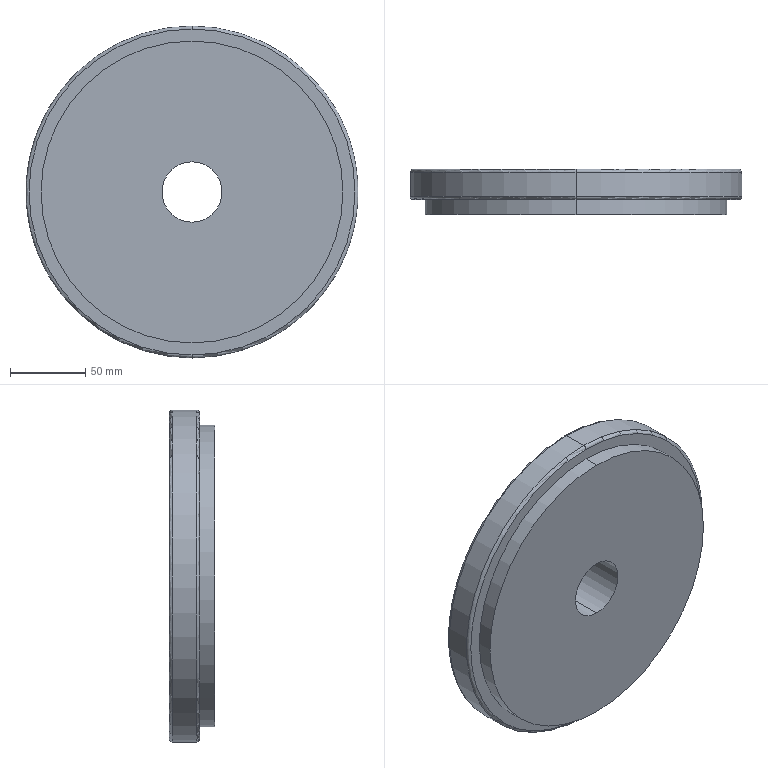Part | SolidWorks | features ICE 2, Extrusion 1, Fillet 1, HoleWzd 1, SketchPattern 1 | 1 solid | 29 faces | box 220 x 30 x 220 mm | volume 1035187 mm3 | cylinder 14 | cone 8 | torus 4 | plane 3 | commonest cylinder face diameters 3.3 x8 40 x2 200 x2 220 x2
STEP:
#1=CARTESIAN_POINT('',(0.,28.,-110.));
#2=VERTEX_POINT('',#1);
#3=CARTESIAN_POINT('',(0.,28.,110.));
#4=VERTEX_POINT('',#3);
#5=CARTESIAN_POINT('',(0.,28.,0.));
#6=DIRECTION('',(0.,-1.,0.));
#7=DIRECTION('',(0.,0.,1.));
#8=AXIS2_PLACEMENT_3D('',#5,#6,#7);
#9=CIRCLE('',#8,110.);
#10=EDGE_CURVE('',#2,#4,#9,.T.);
#11=ORIENTED_EDGE('',*,*,#10,.F.);
#12=CARTESIAN_POINT('',(0.,30.,-108.));
#13=VERTEX_POINT('',#12);
#14=CARTESIAN_POINT('',(0.,28.,-108.));
#15=DIRECTION('',(1.,0.,0.));
#16=DIRECTION('',(0.,0.,-1.));
#17=AXIS2_PLACEMENT_3D('',#14,#15,#16);
#18=CIRCLE('',#17,2.);
#19=EDGE_CURVE('',#2,#13,#18,.T.);
#20=ORIENTED_EDGE('',*,*,#19,.T.);
#21=CARTESIAN_POINT('',(0.,30.,108.));
#22=VERTEX_POINT('',#21);
#23=CARTESIAN_POINT('',(0.,30.,0.));
#24=DIRECTION('',(0.,1.,0.));
#25=DIRECTION('',(0.,0.,1.));
#26=AXIS2_PLACEMENT_3D('',#23,#24,#25);
#27=CIRCLE('',#26,108.);
#28=EDGE_CURVE('',#22,#13,#27,.T.);
#29=ORIENTED_EDGE('',*,*,#28,.F.);
#30=CARTESIAN_POINT('',(0.,28.,108.));
#31=DIRECTION('',(-1.,0.,0.));
#32=DIRECTION('',(0.,0.,1.));
#33=AXIS2_PLACEMENT_3D('',#30,#31,#32);
#34=CIRCLE('',#33,2.);
#35=EDGE_CURVE('',#4,#22,#34,.T.);
#36=ORIENTED_EDGE('',*,*,#35,.F.);
#37=EDGE_LOOP('',(#11,#20,#29,#36));
#38=FACE_OUTER_BOUND('',#37,.T.);
#39=CARTESIAN_POINT('',(0.,28.,0.));
#40=DIRECTION('',(0.,1.,0.));
#41=DIRECTION('',(0.,0.,1.));
#42=AXIS2_PLACEMENT_3D('',#39,#40,#41);
#43=TOROIDAL_SURFACE('',#42,108.,2.);
#44=ADVANCED_FACE('',(#38),#43,.T.);
#45=CARTESIAN_POINT('',(0.,10.,-108.));
#46=VERTEX_POINT('',#45);
#47=CARTESIAN_POINT('',(0.,10.,108.));
#48=VERTEX_POINT('',#47);
#49=CARTESIAN_POINT('',(0.,10.,0.));
#50=DIRECTION('',(0.,-1.,0.));
#51=DIRECTION('',(0.,0.,1.));
#52=AXIS2_PLACEMENT_3D('',#49,#50,#51);
#53=CIRCLE('',#52,108.);
#54=EDGE_CURVE('',#46,#48,#53,.T.);
#55=ORIENTED_EDGE('',*,*,#54,.F.);
#56=CARTESIAN_POINT('',(0.,12.,-110.));
#57=VERTEX_POINT('',#56);
#58=CARTESIAN_POINT('',(0.,12.,-108.));
#59=DIRECTION('',(1.,0.,0.));
#60=DIRECTION('',(0.,0.,-1.));
#61=AXIS2_PLACEMENT_3D('',#58,#59,#60);
#62=CIRCLE('',#61,2.);
#63=EDGE_CURVE('',#46,#57,#62,.T.);
#64=ORIENTED_EDGE('',*,*,#63,.T.);
#65=CARTESIAN_POINT('',(0.,12.,110.));
#66=VERTEX_POINT('',#65);
#67=CARTESIAN_POINT('',(0.,12.,0.));
#68=DIRECTION('',(0.,1.,0.));
#69=DIRECTION('',(0.,0.,1.));
#70=AXIS2_PLACEMENT_3D('',#67,#68,#69);
#71=CIRCLE('',#70,110.);
#72=EDGE_CURVE('',#66,#57,#71,.T.);
#73=ORIENTED_EDGE('',*,*,#72,.F.);
#74=CARTESIAN_POINT('',(0.,12.,108.));
#75=DIRECTION('',(-1.,0.,0.));
#76=DIRECTION('',(0.,0.,1.));
#77=AXIS2_PLACEMENT_3D('',#74,#75,#76);
#78=CIRCLE('',#77,2.);
#79=EDGE_CURVE('',#48,#66,#78,.T.);
#80=ORIENTED_EDGE('',*,*,#79,.F.);
#81=EDGE_LOOP('',(#55,#64,#73,#80));
#82=FACE_OUTER_BOUND('',#81,.T.);
#83=CARTESIAN_POINT('',(0.,12.,0.));
#84=DIRECTION('',(0.,1.,0.));
#85=DIRECTION('',(0.,0.,1.));
#86=AXIS2_PLACEMENT_3D('',#83,#84,#85);
#87=TOROIDAL_SURFACE('',#86,108.,2.);
#88=ADVANCED_FACE('',(#82),#87,.T.);
#89=CARTESIAN_POINT('',(-22.707,19.9,-12.11));
#90=VERTEX_POINT('',#89);
#91=CARTESIAN_POINT('',(-22.707,19.9,-8.81));
#92=VERTEX_POINT('',#91);
#93=CARTESIAN_POINT('',(-22.707,19.9,-10.46));
#94=DIRECTION('',(0.,1.,0.));
#95=DIRECTION('',(0.,0.,1.));
#96=AXIS2_PLACEMENT_3D('',#93,#94,#95);
#97=CIRCLE('',#96,1.65);
#98=EDGE_CURVE('',#90,#92,#97,.T.);
#99=ORIENTED_EDGE('',*,*,#98,.F.);
#100=CARTESIAN_POINT('',(-22.707,30.,-12.11));
#101=VERTEX_POINT('',#100);
#102=CARTESIAN_POINT('',(-22.707,30.,-12.11));
#103=DIRECTION('',(0.,1.,0.));
#104=VECTOR('',#103,1000.);
#105=LINE('',#102,#104);
#106=EDGE_CURVE('',#90,#101,#105,.T.);
#107=ORIENTED_EDGE('',*,*,#106,.T.);
#108=CARTESIAN_POINT('',(-22.707,30.,-8.81));
#109=VERTEX_POINT('',#108);
#110=CARTESIAN_POINT('',(-22.707,30.,-10.46));
#111=DIRECTION('',(0.,1.,0.));
#112=DIRECTION('',(0.,0.,1.));
#113=AXIS2_PLACEMENT_3D('',#110,#111,#112);
#114=CIRCLE('',#113,1.65);
#115=EDGE_CURVE('',#101,#109,#114,.T.);
#116=ORIENTED_EDGE('',*,*,#115,.T.);
#117=CARTESIAN_POINT('',(-22.707,30.,-8.81));
#118=DIRECTION('',(0.,1.,0.));
#119=VECTOR('',#118,1000.);
#120=LINE('',#117,#119);
#121=EDGE_CURVE('',#92,#109,#120,.T.);
#122=ORIENTED_EDGE('',*,*,#121,.F.);
#123=EDGE_LOOP('',(#99,#107,#116,#122));
#124=FACE_OUTER_BOUND('',#123,.T.);
#125=CARTESIAN_POINT('',(-22.707,30.,-10.46));
#126=DIRECTION('',(0.,1.,0.));
#127=DIRECTION('',(0.,0.,1.));
#128=AXIS2_PLACEMENT_3D('',#125,#126,#127);
#129=CYLINDRICAL_SURFACE('',#128,1.65);
#130=ADVANCED_FACE('',(#124),#129,.F.);
#131=CARTESIAN_POINT('',(-22.707,18.909,-10.46));
#132=VERTEX_POINT('',#131);
#133=CARTESIAN_POINT('',(-22.707,19.9,-8.81));
#134=DIRECTION('',(0.,0.515,0.8572));
#135=VECTOR('',#134,1000.);
#136=LINE('',#133,#135);
#137=EDGE_CURVE('',#132,#92,#136,.T.);
#138=ORIENTED_EDGE('',*,*,#137,.F.);
#139=CARTESIAN_POINT('',(-22.707,19.9,-12.11));
#140=DIRECTION('',(0.,0.515,-0.8572));
#141=VECTOR('',#140,1000.);
#142=LINE('',#139,#141);
#143=EDGE_CURVE('',#132,#90,#142,.T.);
#144=ORIENTED_EDGE('',*,*,#143,.T.);
#145=ORIENTED_EDGE('',*,*,#98,.T.);
#146=EDGE_LOOP('',(#138,#144,#145));
#147=FACE_OUTER_BOUND('',#146,.T.);
#148=CARTESIAN_POINT('',(-22.707,19.9,-10.46));
#149=DIRECTION('',(0.,1.,0.));
#150=DIRECTION('',(0.,0.,1.));
#151=AXIS2_PLACEMENT_3D('',#148,#149,#150);
#152=CONICAL_SURFACE('',#151,1.65,1.03);
#153=ADVANCED_FACE('',(#147),#152,.F.);
#154=CARTESIAN_POINT('',(-7.031,19.9,30.343));
#155=VERTEX_POINT('',#154);
#156=CARTESIAN_POINT('',(-7.031,19.9,33.643));
#157=VERTEX_POINT('',#156);
#158=CARTESIAN_POINT('',(-7.031,19.9,31.993));
#159=DIRECTION('',(0.,1.,0.));
#160=DIRECTION('',(0.,0.,1.));
#161=AXIS2_PLACEMENT_3D('',#158,#159,#160);
#162=CIRCLE('',#161,1.65);
#163=EDGE_CURVE('',#155,#157,#162,.T.);
#164=ORIENTED_EDGE('',*,*,#163,.F.);
#165=CARTESIAN_POINT('',(-7.031,30.,30.343));
#166=VERTEX_POINT('',#165);
#167=CARTESIAN_POINT('',(-7.031,30.,30.343));
#168=DIRECTION('',(0.,1.,0.));
#169=VECTOR('',#168,1000.);
#170=LINE('',#167,#169);
#171=EDGE_CURVE('',#155,#166,#170,.T.);
#172=ORIENTED_EDGE('',*,*,#171,.T.);
#173=CARTESIAN_POINT('',(-7.031,30.,33.643));
#174=VERTEX_POINT('',#173);
#175=CARTESIAN_POINT('',(-7.031,30.,31.993));
#176=DIRECTION('',(0.,1.,0.));
#177=DIRECTION('',(0.,0.,1.));
#178=AXIS2_PLACEMENT_3D('',#175,#176,#177);
#179=CIRCLE('',#178,1.65);
#180=EDGE_CURVE('',#166,#174,#179,.T.);
#181=ORIENTED_EDGE('',*,*,#180,.T.);
#182=CARTESIAN_POINT('',(-7.031,30.,33.643));
#183=DIRECTION('',(0.,1.,0.));
#184=VECTOR('',#183,1000.);
#185=LINE('',#182,#184);
#186=EDGE_CURVE('',#157,#174,#185,.T.);
#187=ORIENTED_EDGE('',*,*,#186,.F.);
#188=EDGE_LOOP('',(#164,#172,#181,#187));
#189=FACE_OUTER_BOUND('',#188,.T.);
#190=CARTESIAN_POINT('',(-7.031,30.,31.993));
#191=DIRECTION('',(0.,1.,0.));
#192=DIRECTION('',(0.,0.,1.));
#193=AXIS2_PLACEMENT_3D('',#190,#191,#192);
#194=CYLINDRICAL_SURFACE('',#193,1.65);
#195=ADVANCED_FACE('',(#189),#194,.F.);
#196=CARTESIAN_POINT('',(-7.031,18.909,31.993));
#197=VERTEX_POINT('',#196);
#198=CARTESIAN_POINT('',(-7.031,19.9,33.643));
#199=DIRECTION('',(0.,0.515,0.8572));
#200=VECTOR('',#199,1000.);
#201=LINE('',#198,#200);
#202=EDGE_CURVE('',#197,#157,#201,.T.);
#203=ORIENTED_EDGE('',*,*,#202,.F.);
#204=CARTESIAN_POINT('',(-7.031,19.9,30.343));
#205=DIRECTION('',(0.,0.515,-0.8572));
#206=VECTOR('',#205,1000.);
#207=LINE('',#204,#206);
#208=EDGE_CURVE('',#197,#155,#207,.T.);
#209=ORIENTED_EDGE('',*,*,#208,.T.);
#210=ORIENTED_EDGE('',*,*,#163,.T.);
#211=EDGE_LOOP('',(#203,#209,#210));
#212=FACE_OUTER_BOUND('',#211,.T.);
#213=CARTESIAN_POINT('',(-7.031,19.9,31.993));
#214=DIRECTION('',(0.,1.,0.));
#215=DIRECTION('',(0.,0.,1.));
#216=AXIS2_PLACEMENT_3D('',#213,#214,#215);
#217=CONICAL_SURFACE('',#216,1.65,1.03);
#218=ADVANCED_FACE('',(#212),#217,.F.);
#219=CARTESIAN_POINT('',(35.422,19.9,14.668));
#220=VERTEX_POINT('',#219);
#221=CARTESIAN_POINT('',(35.422,19.9,17.968));
#222=VERTEX_POINT('',#221);
#223=CARTESIAN_POINT('',(35.422,19.9,16.318));
#224=DIRECTION('',(0.,1.,0.));
#225=DIRECTION('',(0.,0.,1.));
#226=AXIS2_PLACEMENT_3D('',#223,#224,#225);
#227=CIRCLE('',#226,1.65);
#228=EDGE_CURVE('',#220,#222,#227,.T.);
#229=ORIENTED_EDGE('',*,*,#228,.F.);
#230=CARTESIAN_POINT('',(35.422,30.,14.668));
#231=VERTEX_POINT('',#230);
#232=CARTESIAN_POINT('',(35.422,30.,14.668));
#233=DIRECTION('',(0.,1.,0.));
#234=VECTOR('',#233,1000.);
#235=LINE('',#232,#234);
#236=EDGE_CURVE('',#220,#231,#235,.T.);
#237=ORIENTED_EDGE('',*,*,#236,.T.);
#238=CARTESIAN_POINT('',(35.422,30.,17.968));
#239=VERTEX_POINT('',#238);
#240=CARTESIAN_POINT('',(35.422,30.,16.318));
#241=DIRECTION('',(0.,1.,0.));
#242=DIRECTION('',(0.,0.,1.));
#243=AXIS2_PLACEMENT_3D('',#240,#241,#242);
#244=CIRCLE('',#243,1.65);
#245=EDGE_CURVE('',#231,#239,#244,.T.);
#246=ORIENTED_EDGE('',*,*,#245,.T.);
#247=CARTESIAN_POINT('',(35.422,30.,17.968));
#248=DIRECTION('',(0.,1.,0.));
#249=VECTOR('',#248,1000.);
#250=LINE('',#247,#249);
#251=EDGE_CURVE('',#222,#239,#250,.T.);
#252=ORIENTED_EDGE('',*,*,#251,.F.);
#253=EDGE_LOOP('',(#229,#237,#246,#252));
#254=FACE_OUTER_BOUND('',#253,.T.);
#255=CARTESIAN_POINT('',(35.422,30.,16.318));
#256=DIRECTION('',(0.,1.,0.));
#257=DIRECTION('',(0.,0.,1.));
#258=AXIS2_PLACEMENT_3D('',#255,#256,#257);
#259=CYLINDRICAL_SURFACE('',#258,1.65);
#260=ADVANCED_FACE('',(#254),#259,.F.);
#261=CARTESIAN_POINT('',(35.422,18.909,16.318));
#262=VERTEX_POINT('',#261);
#263=CARTESIAN_POINT('',(35.422,19.9,17.968));
#264=DIRECTION('',(0.,0.515,0.8572));
#265=VECTOR('',#264,1000.);
#266=LINE('',#263,#265);
#267=EDGE_CURVE('',#262,#222,#266,.T.);
#268=ORIENTED_EDGE('',*,*,#267,.F.);
#269=CARTESIAN_POINT('',(35.422,19.9,14.668));
#270=DIRECTION('',(0.,0.515,-0.8572));
#271=VECTOR('',#270,1000.);
#272=LINE('',#269,#271);
#273=EDGE_CURVE('',#262,#220,#272,.T.);
#274=ORIENTED_EDGE('',*,*,#273,.T.);
#275=ORIENTED_EDGE('',*,*,#228,.T.);
#276=EDGE_LOOP('',(#268,#274,#275));
#277=FACE_OUTER_BOUND('',#276,.T.);
#278=CARTESIAN_POINT('',(35.422,19.9,16.318));
#279=DIRECTION('',(0.,1.,0.));
#280=DIRECTION('',(0.,0.,1.));
#281=AXIS2_PLACEMENT_3D('',#278,#279,#280);
#282=CONICAL_SURFACE('',#281,1.65,1.03);
#283=ADVANCED_FACE('',(#277),#282,.F.);
#284=CARTESIAN_POINT('',(19.747,19.9,-27.786));
#285=VERTEX_POINT('',#284);
#286=CARTESIAN_POINT('',(19.747,19.9,-24.486));
#287=VERTEX_POINT('',#286);
#288=CARTESIAN_POINT('',(19.747,19.9,-26.136));
#289=DIRECTION('',(0.,1.,0.));
#290=DIRECTION('',(0.,0.,1.));
#291=AXIS2_PLACEMENT_3D('',#288,#289,#290);
#292=CIRCLE('',#291,1.65);
#293=EDGE_CURVE('',#285,#287,#292,.T.);
#294=ORIENTED_EDGE('',*,*,#293,.F.);
#295=CARTESIAN_POINT('',(19.747,30.,-27.786));
#296=VERTEX_POINT('',#295);
#297=CARTESIAN_POINT('',(19.747,30.,-27.786));
#298=DIRECTION('',(0.,1.,0.));
#299=VECTOR('',#298,1000.);
#300=LINE('',#297,#299);
#301=EDGE_CURVE('',#285,#296,#300,.T.);
#302=ORIENTED_EDGE('',*,*,#301,.T.);
#303=CARTESIAN_POINT('',(19.747,30.,-24.486));
#304=VERTEX_POINT('',#303);
#305=CARTESIAN_POINT('',(19.747,30.,-26.136));
#306=DIRECTION('',(0.,1.,0.));
#307=DIRECTION('',(0.,0.,1.));
#308=AXIS2_PLACEMENT_3D('',#305,#306,#307);
#309=CIRCLE('',#308,1.65);
#310=EDGE_CURVE('',#296,#304,#309,.T.);
#311=ORIENTED_EDGE('',*,*,#310,.T.);
#312=CARTESIAN_POINT('',(19.747,30.,-24.486));
#313=DIRECTION('',(0.,1.,0.));
#314=VECTOR('',#313,1000.);
#315=LINE('',#312,#314);
#316=EDGE_CURVE('',#287,#304,#315,.T.);
#317=ORIENTED_EDGE('',*,*,#316,.F.);
#318=EDGE_LOOP('',(#294,#302,#311,#317));
#319=FACE_OUTER_BOUND('',#318,.T.);
#320=CARTESIAN_POINT('',(19.747,30.,-26.136));
#321=DIRECTION('',(0.,1.,0.));
#322=DIRECTION('',(0.,0.,1.));
#323=AXIS2_PLACEMENT_3D('',#320,#321,#322);
#324=CYLINDRICAL_SURFACE('',#323,1.65);
#325=ADVANCED_FACE('',(#319),#324,.F.);
#326=CARTESIAN_POINT('',(19.747,18.909,-26.136));
#327=VERTEX_POINT('',#326);
#328=CARTESIAN_POINT('',(19.747,19.9,-24.486));
#329=DIRECTION('',(0.,0.515,0.8572));
#330=VECTOR('',#329,1000.);
#331=LINE('',#328,#330);
#332=EDGE_CURVE('',#327,#287,#331,.T.);
#333=ORIENTED_EDGE('',*,*,#332,.F.);
#334=CARTESIAN_POINT('',(19.747,19.9,-27.786));
#335=DIRECTION('',(0.,0.515,-0.8572));
#336=VECTOR('',#335,1000.);
#337=LINE('',#334,#336);
#338=EDGE_CURVE('',#327,#285,#337,.T.);
#339=ORIENTED_EDGE('',*,*,#338,.T.);
#340=ORIENTED_EDGE('',*,*,#293,.T.);
#341=EDGE_LOOP('',(#333,#339,#340));
#342=FACE_OUTER_BOUND('',#341,.T.);
#343=CARTESIAN_POINT('',(19.747,19.9,-26.136));
#344=DIRECTION('',(0.,1.,0.));
#345=DIRECTION('',(0.,0.,1.));
#346=AXIS2_PLACEMENT_3D('',#343,#344,#345);
#347=CONICAL_SURFACE('',#346,1.65,1.03);
#348=ADVANCED_FACE('',(#342),#347,.F.);
#349=CARTESIAN_POINT('',(0.,0.,-20.));
#350=VERTEX_POINT('',#349);
#351=CARTESIAN_POINT('',(0.,0.,20.));
#352=VERTEX_POINT('',#351);
#353=CARTESIAN_POINT('',(0.,0.,0.));
#354=DIRECTION('',(0.,1.,0.));
#355=DIRECTION('',(0.,0.,1.));
#356=AXIS2_PLACEMENT_3D('',#353,#354,#355);
#357=CIRCLE('',#356,20.);
#358=EDGE_CURVE('',#350,#352,#357,.T.);
#359=ORIENTED_EDGE('',*,*,#358,.F.);
#360=CARTESIAN_POINT('',(0.,30.,-20.));
#361=VERTEX_POINT('',#360);
#362=CARTESIAN_POINT('',(0.,0.,-20.));
#363=DIRECTION('',(0.,1.,0.));
#364=VECTOR('',#363,1000.);
#365=LINE('',#362,#364);
#366=EDGE_CURVE('',#350,#361,#365,.T.);
#367=ORIENTED_EDGE('',*,*,#366,.T.);
#368=CARTESIAN_POINT('',(0.,30.,20.));
#369=VERTEX_POINT('',#368);
#370=CARTESIAN_POINT('',(0.,30.,0.));
#371=DIRECTION('',(0.,1.,0.));
#372=DIRECTION('',(0.,0.,1.));
#373=AXIS2_PLACEMENT_3D('',#370,#371,#372);
#374=CIRCLE('',#373,20.);
#375=EDGE_CURVE('',#361,#369,#374,.T.);
#376=ORIENTED_EDGE('',*,*,#375,.T.);
#377=CARTESIAN_POINT('',(0.,0.,20.));
#378=DIRECTION('',(0.,1.,0.));
#379=VECTOR('',#378,1000.);
#380=LINE('',#377,#379);
#381=EDGE_CURVE('',#352,#369,#380,.T.);
#382=ORIENTED_EDGE('',*,*,#381,.F.);
#383=EDGE_LOOP('',(#359,#367,#376,#382));
#384=FACE_OUTER_BOUND('',#383,.T.);
#385=CARTESIAN_POINT('',(0.,0.,0.));
#386=DIRECTION('',(0.,1.,0.));
#387=DIRECTION('',(0.,0.,1.));
#388=AXIS2_PLACEMENT_3D('',#385,#386,#387);
#389=CYLINDRICAL_SURFACE('',#388,20.);
#390=ADVANCED_FACE('',(#384),#389,.F.);
#391=ORIENTED_EDGE('',*,*,#10,.T.);
#392=CARTESIAN_POINT('',(0.,30.,110.));
#393=DIRECTION('',(0.,-1.,0.));
#394=VECTOR('',#393,1000.);
#395=LINE('',#392,#394);
#396=EDGE_CURVE('',#4,#66,#395,.T.);
#397=ORIENTED_EDGE('',*,*,#396,.T.);
#398=ORIENTED_EDGE('',*,*,#72,.T.);
#399=CARTESIAN_POINT('',(0.,30.,-110.));
#400=DIRECTION('',(0.,-1.,0.));
#401=VECTOR('',#400,1000.);
#402=LINE('',#399,#401);
#403=EDGE_CURVE('',#2,#57,#402,.T.);
#404=ORIENTED_EDGE('',*,*,#403,.F.);
#405=EDGE_LOOP('',(#391,#397,#398,#404));
#406=FACE_OUTER_BOUND('',#405,.T.);
#407=CARTESIAN_POINT('',(0.,30.,0.));
#408=DIRECTION('',(0.,-1.,0.));
#409=DIRECTION('',(0.,0.,-1.));
#410=AXIS2_PLACEMENT_3D('',#407,#408,#409);
#411=CYLINDRICAL_SURFACE('',#410,110.);
#412=ADVANCED_FACE('',(#406),#411,.T.);
#413=CARTESIAN_POINT('',(0.,10.,100.));
#414=VERTEX_POINT('',#413);
#415=CARTESIAN_POINT('',(0.,10.,-100.));
#416=VERTEX_POINT('',#415);
#417=CARTESIAN_POINT('',(0.,10.,0.));
#418=DIRECTION('',(0.,1.,0.));
#419=DIRECTION('',(0.,0.,1.));
#420=AXIS2_PLACEMENT_3D('',#417,#418,#419);
#421=CIRCLE('',#420,100.);
#422=EDGE_CURVE('',#414,#416,#421,.T.);
#423=ORIENTED_EDGE('',*,*,#422,.F.);
#424=CARTESIAN_POINT('',(0.,0.,100.));
#425=VERTEX_POINT('',#424);
#426=CARTESIAN_POINT('',(0.,10.,100.));
#427=DIRECTION('',(0.,-1.,0.));
#428=VECTOR('',#427,1000.);
#429=LINE('',#426,#428);
#430=EDGE_CURVE('',#414,#425,#429,.T.);
#431=ORIENTED_EDGE('',*,*,#430,.T.);
#432=CARTESIAN_POINT('',(0.,0.,-100.));
#433=VERTEX_POINT('',#432);
#434=CARTESIAN_POINT('',(0.,0.,0.));
#435=DIRECTION('',(0.,1.,0.));
#436=DIRECTION('',(0.,0.,1.));
#437=AXIS2_PLACEMENT_3D('',#434,#435,#436);
#438=CIRCLE('',#437,100.);
#439=EDGE_CURVE('',#425,#433,#438,.T.);
#440=ORIENTED_EDGE('',*,*,#439,.T.);
#441=CARTESIAN_POINT('',(0.,10.,-100.));
#442=DIRECTION('',(0.,-1.,0.));
#443=VECTOR('',#442,1000.);
#444=LINE('',#441,#443);
#445=EDGE_CURVE('',#416,#433,#444,.T.);
#446=ORIENTED_EDGE('',*,*,#445,.F.);
#447=EDGE_LOOP('',(#423,#431,#440,#446));
#448=FACE_OUTER_BOUND('',#447,.T.);
#449=CARTESIAN_POINT('',(0.,10.,0.));
#450=DIRECTION('',(0.,-1.,0.));
#451=DIRECTION('',(0.,0.,-1.));
#452=AXIS2_PLACEMENT_3D('',#449,#450,#451);
#453=CYLINDRICAL_SURFACE('',#452,100.);
#454=ADVANCED_FACE('',(#448),#453,.T.);
#455=ORIENTED_EDGE('',*,*,#430,.F.);
#456=CARTESIAN_POINT('',(0.,10.,0.));
#457=DIRECTION('',(0.,1.,0.));
#458=DIRECTION('',(0.,0.,1.));
#459=AXIS2_PLACEMENT_3D('',#456,#457,#458);
#460=CIRCLE('',#459,100.);
#461=EDGE_CURVE('',#416,#414,#460,.T.);
#462=ORIENTED_EDGE('',*,*,#461,.F.);
#463=ORIENTED_EDGE('',*,*,#445,.T.);
#464=CARTESIAN_POINT('',(0.,0.,0.));
#465=DIRECTION('',(0.,1.,0.));
#466=DIRECTION('',(0.,0.,1.));
#467=AXIS2_PLACEMENT_3D('',#464,#465,#466);
#468=CIRCLE('',#467,100.);
#469=EDGE_CURVE('',#433,#425,#468,.T.);
#470=ORIENTED_EDGE('',*,*,#469,.T.);
#471=EDGE_LOOP('',(#455,#462,#463,#470));
#472=FACE_OUTER_BOUND('',#471,.T.);
#473=CARTESIAN_POINT('',(0.,10.,0.));
#474=DIRECTION('',(0.,-1.,0.));
#475=DIRECTION('',(0.,0.,-1.));
#476=AXIS2_PLACEMENT_3D('',#473,#474,#475);
#477=CYLINDRICAL_SURFACE('',#476,100.);
#478=ADVANCED_FACE('',(#472),#477,.T.);
#479=CARTESIAN_POINT('',(0.,0.,0.));
#480=DIRECTION('',(0.,1.,0.));
#481=DIRECTION('',(0.,0.,1.));
#482=AXIS2_PLACEMENT_3D('',#479,#480,#481);
#483=CIRCLE('',#482,20.);
#484=EDGE_CURVE('',#352,#350,#483,.T.);
#485=ORIENTED_EDGE('',*,*,#484,.T.);
#486=ORIENTED_EDGE('',*,*,#358,.T.);
#487=EDGE_LOOP('',(#485,#486));
#488=FACE_BOUND('',#487,.T.);
#489=ORIENTED_EDGE('',*,*,#469,.F.);
#490=ORIENTED_EDGE('',*,*,#439,.F.);
#491=EDGE_LOOP('',(#489,#490));
#492=FACE_OUTER_BOUND('',#491,.T.);
#493=CARTESIAN_POINT('',(0.,0.,0.));
#494=DIRECTION('',(0.,1.,0.));
#495=DIRECTION('',(0.,0.,1.));
#496=AXIS2_PLACEMENT_3D('',#493,#494,#495);
#497=PLANE('',#496);
#498=ADVANCED_FACE('',(#488,#492),#497,.F.);
#499=ORIENTED_EDGE('',*,*,#396,.F.);
#500=CARTESIAN_POINT('',(0.,28.,0.));
#501=DIRECTION('',(0.,-1.,0.));
#502=DIRECTION('',(0.,0.,1.));
#503=AXIS2_PLACEMENT_3D('',#500,#501,#502);
#504=CIRCLE('',#503,110.);
#505=EDGE_CURVE('',#4,#2,#504,.T.);
#506=ORIENTED_EDGE('',*,*,#505,.T.);
#507=ORIENTED_EDGE('',*,*,#403,.T.);
#508=CARTESIAN_POINT('',(0.,12.,0.));
#509=DIRECTION('',(0.,1.,0.));
#510=DIRECTION('',(0.,0.,1.));
#511=AXIS2_PLACEMENT_3D('',#508,#509,#510);
#512=CIRCLE('',#511,110.);
#513=EDGE_CURVE('',#57,#66,#512,.T.);
#514=ORIENTED_EDGE('',*,*,#513,.T.);
#515=EDGE_LOOP('',(#499,#506,#507,#514));
#516=FACE_OUTER_BOUND('',#515,.T.);
#517=CARTESIAN_POINT('',(0.,30.,0.));
#518=DIRECTION('',(0.,-1.,0.));
#519=DIRECTION('',(0.,0.,-1.));
#520=AXIS2_PLACEMENT_3D('',#517,#518,#519);
#521=CYLINDRICAL_SURFACE('',#520,110.);
#522=ADVANCED_FACE('',(#516),#521,.T.);
#523=ORIENTED_EDGE('',*,*,#28,.T.);
#524=CARTESIAN_POINT('',(0.,30.,0.));
#525=DIRECTION('',(0.,1.,0.));
#526=DIRECTION('',(0.,0.,1.));
#527=AXIS2_PLACEMENT_3D('',#524,#525,#526);
#528=CIRCLE('',#527,108.);
#529=EDGE_CURVE('',#13,#22,#528,.T.);
#530=ORIENTED_EDGE('',*,*,#529,.T.);
#531=EDGE_LOOP('',(#523,#530));
#532=FACE_OUTER_BOUND('',#531,.T.);
#533=CARTESIAN_POINT('',(-22.707,30.,-10.46));
#534=DIRECTION('',(0.,1.,0.));
#535=DIRECTION('',(0.,0.,1.));
#536=AXIS2_PLACEMENT_3D('',#533,#534,#535);
#537=CIRCLE('',#536,1.65);
#538=EDGE_CURVE('',#109,#101,#537,.T.);
#539=ORIENTED_EDGE('',*,*,#538,.F.);
#540=ORIENTED_EDGE('',*,*,#115,.F.);
#541=EDGE_LOOP('',(#539,#540));
#542=FACE_BOUND('',#541,.T.);
#543=CARTESIAN_POINT('',(-7.031,30.,31.993));
#544=DIRECTION('',(0.,1.,0.));
#545=DIRECTION('',(0.,0.,1.));
#546=AXIS2_PLACEMENT_3D('',#543,#544,#545);
#547=CIRCLE('',#546,1.65);
#548=EDGE_CURVE('',#174,#166,#547,.T.);
#549=ORIENTED_EDGE('',*,*,#548,.F.);
#550=ORIENTED_EDGE('',*,*,#180,.F.);
#551=EDGE_LOOP('',(#549,#550));
#552=FACE_BOUND('',#551,.T.);
#553=CARTESIAN_POINT('',(35.422,30.,16.318));
#554=DIRECTION('',(0.,1.,0.));
#555=DIRECTION('',(0.,0.,1.));
#556=AXIS2_PLACEMENT_3D('',#553,#554,#555);
#557=CIRCLE('',#556,1.65);
#558=EDGE_CURVE('',#239,#231,#557,.T.);
#559=ORIENTED_EDGE('',*,*,#558,.F.);
#560=ORIENTED_EDGE('',*,*,#245,.F.);
#561=EDGE_LOOP('',(#559,#560));
#562=FACE_BOUND('',#561,.T.);
#563=CARTESIAN_POINT('',(19.747,30.,-26.136));
#564=DIRECTION('',(0.,1.,0.));
#565=DIRECTION('',(0.,0.,1.));
#566=AXIS2_PLACEMENT_3D('',#563,#564,#565);
#567=CIRCLE('',#566,1.65);
#568=EDGE_CURVE('',#304,#296,#567,.T.);
#569=ORIENTED_EDGE('',*,*,#568,.F.);
#570=ORIENTED_EDGE('',*,*,#310,.F.);
#571=EDGE_LOOP('',(#569,#570));
#572=FACE_BOUND('',#571,.T.);
#573=CARTESIAN_POINT('',(0.,30.,0.));
#574=DIRECTION('',(0.,1.,0.));
#575=DIRECTION('',(0.,0.,1.));
#576=AXIS2_PLACEMENT_3D('',#573,#574,#575);
#577=CIRCLE('',#576,20.);
#578=EDGE_CURVE('',#369,#361,#577,.T.);
#579=ORIENTED_EDGE('',*,*,#578,.F.);
#580=ORIENTED_EDGE('',*,*,#375,.F.);
#581=EDGE_LOOP('',(#579,#580));
#582=FACE_BOUND('',#581,.T.);
#583=CARTESIAN_POINT('',(0.,30.,0.));
#584=DIRECTION('',(0.,1.,0.));
#585=DIRECTION('',(0.,0.,1.));
#586=AXIS2_PLACEMENT_3D('',#583,#584,#585);
#587=PLANE('',#586);
#588=ADVANCED_FACE('',(#532,#542,#552,#562,#572,#582),#587,.T.);
#589=CARTESIAN_POINT('',(0.,10.,0.));
#590=DIRECTION('',(0.,-1.,0.));
#591=DIRECTION('',(0.,0.,1.));
#592=AXIS2_PLACEMENT_3D('',#589,#590,#591);
#593=CIRCLE('',#592,108.);
#594=EDGE_CURVE('',#48,#46,#593,.T.);
#595=ORIENTED_EDGE('',*,*,#594,.T.);
#596=ORIENTED_EDGE('',*,*,#54,.T.);
#597=EDGE_LOOP('',(#595,#596));
#598=FACE_OUTER_BOUND('',#597,.T.);
#599=ORIENTED_EDGE('',*,*,#461,.T.);
#600=ORIENTED_EDGE('',*,*,#422,.T.);
#601=EDGE_LOOP('',(#599,#600));
#602=FACE_BOUND('',#601,.T.);
#603=CARTESIAN_POINT('',(0.,10.,0.));
#604=DIRECTION('',(0.,1.,0.));
#605=DIRECTION('',(0.,0.,1.));
#606=AXIS2_PLACEMENT_3D('',#603,#604,#605);
#607=PLANE('',#606);
#608=ADVANCED_FACE('',(#598,#602),#607,.F.);
#609=ORIENTED_EDGE('',*,*,#366,.F.);
#610=ORIENTED_EDGE('',*,*,#484,.F.);
#611=ORIENTED_EDGE('',*,*,#381,.T.);
#612=ORIENTED_EDGE('',*,*,#578,.T.);
#613=EDGE_LOOP('',(#609,#610,#611,#612));
#614=FACE_OUTER_BOUND('',#613,.T.);
#615=CARTESIAN_POINT('',(0.,0.,0.));
#616=DIRECTION('',(0.,1.,0.));
#617=DIRECTION('',(0.,0.,1.));
#618=AXIS2_PLACEMENT_3D('',#615,#616,#617);
#619=CYLINDRICAL_SURFACE('',#618,20.);
#620=ADVANCED_FACE('',(#614),#619,.F.);
#621=ORIENTED_EDGE('',*,*,#338,.F.);
#622=ORIENTED_EDGE('',*,*,#332,.T.);
#623=CARTESIAN_POINT('',(19.747,19.9,-26.136));
#624=DIRECTION('',(0.,1.,0.));
#625=DIRECTION('',(0.,0.,1.));
#626=AXIS2_PLACEMENT_3D('',#623,#624,#625);
#627=CIRCLE('',#626,1.65);
#628=EDGE_CURVE('',#287,#285,#627,.T.);
#629=ORIENTED_EDGE('',*,*,#628,.T.);
#630=EDGE_LOOP('',(#621,#622,#629));
#631=FACE_OUTER_BOUND('',#630,.T.);
#632=CARTESIAN_POINT('',(19.747,19.9,-26.136));
#633=DIRECTION('',(0.,1.,0.));
#634=DIRECTION('',(0.,0.,1.));
#635=AXIS2_PLACEMENT_3D('',#632,#633,#634);
#636=CONICAL_SURFACE('',#635,1.65,1.03);
#637=ADVANCED_FACE('',(#631),#636,.F.);
#638=ORIENTED_EDGE('',*,*,#301,.F.);
#639=ORIENTED_EDGE('',*,*,#628,.F.);
#640=ORIENTED_EDGE('',*,*,#316,.T.);
#641=ORIENTED_EDGE('',*,*,#568,.T.);
#642=EDGE_LOOP('',(#638,#639,#640,#641));
#643=FACE_OUTER_BOUND('',#642,.T.);
#644=CARTESIAN_POINT('',(19.747,30.,-26.136));
#645=DIRECTION('',(0.,1.,0.));
#646=DIRECTION('',(0.,0.,1.));
#647=AXIS2_PLACEMENT_3D('',#644,#645,#646);
#648=CYLINDRICAL_SURFACE('',#647,1.65);
#649=ADVANCED_FACE('',(#643),#648,.F.);
#650=ORIENTED_EDGE('',*,*,#273,.F.);
#651=ORIENTED_EDGE('',*,*,#267,.T.);
#652=CARTESIAN_POINT('',(35.422,19.9,16.318));
#653=DIRECTION('',(0.,1.,0.));
#654=DIRECTION('',(0.,0.,1.));
#655=AXIS2_PLACEMENT_3D('',#652,#653,#654);
#656=CIRCLE('',#655,1.65);
#657=EDGE_CURVE('',#222,#220,#656,.T.);
#658=ORIENTED_EDGE('',*,*,#657,.T.);
#659=EDGE_LOOP('',(#650,#651,#658));
#660=FACE_OUTER_BOUND('',#659,.T.);
#661=CARTESIAN_POINT('',(35.422,19.9,16.318));
#662=DIRECTION('',(0.,1.,0.));
#663=DIRECTION('',(0.,0.,1.));
#664=AXIS2_PLACEMENT_3D('',#661,#662,#663);
#665=CONICAL_SURFACE('',#664,1.65,1.03);
#666=ADVANCED_FACE('',(#660),#665,.F.);
#667=ORIENTED_EDGE('',*,*,#236,.F.);
#668=ORIENTED_EDGE('',*,*,#657,.F.);
#669=ORIENTED_EDGE('',*,*,#251,.T.);
#670=ORIENTED_EDGE('',*,*,#558,.T.);
#671=EDGE_LOOP('',(#667,#668,#669,#670));
#672=FACE_OUTER_BOUND('',#671,.T.);
#673=CARTESIAN_POINT('',(35.422,30.,16.318));
#674=DIRECTION('',(0.,1.,0.));
#675=DIRECTION('',(0.,0.,1.));
#676=AXIS2_PLACEMENT_3D('',#673,#674,#675);
#677=CYLINDRICAL_SURFACE('',#676,1.65);
#678=ADVANCED_FACE('',(#672),#677,.F.);
#679=ORIENTED_EDGE('',*,*,#208,.F.);
#680=ORIENTED_EDGE('',*,*,#202,.T.);
#681=CARTESIAN_POINT('',(-7.031,19.9,31.993));
#682=DIRECTION('',(0.,1.,0.));
#683=DIRECTION('',(0.,0.,1.));
#684=AXIS2_PLACEMENT_3D('',#681,#682,#683);
#685=CIRCLE('',#684,1.65);
#686=EDGE_CURVE('',#157,#155,#685,.T.);
#687=ORIENTED_EDGE('',*,*,#686,.T.);
#688=EDGE_LOOP('',(#679,#680,#687));
#689=FACE_OUTER_BOUND('',#688,.T.);
#690=CARTESIAN_POINT('',(-7.031,19.9,31.993));
#691=DIRECTION('',(0.,1.,0.));
#692=DIRECTION('',(0.,0.,1.));
#693=AXIS2_PLACEMENT_3D('',#690,#691,#692);
#694=CONICAL_SURFACE('',#693,1.65,1.03);
#695=ADVANCED_FACE('',(#689),#694,.F.);
#696=ORIENTED_EDGE('',*,*,#171,.F.);
#697=ORIENTED_EDGE('',*,*,#686,.F.);
#698=ORIENTED_EDGE('',*,*,#186,.T.);
#699=ORIENTED_EDGE('',*,*,#548,.T.);
#700=EDGE_LOOP('',(#696,#697,#698,#699));
#701=FACE_OUTER_BOUND('',#700,.T.);
#702=CARTESIAN_POINT('',(-7.031,30.,31.993));
#703=DIRECTION('',(0.,1.,0.));
#704=DIRECTION('',(0.,0.,1.));
#705=AXIS2_PLACEMENT_3D('',#702,#703,#704);
#706=CYLINDRICAL_SURFACE('',#705,1.65);
#707=ADVANCED_FACE('',(#701),#706,.F.);
#708=ORIENTED_EDGE('',*,*,#143,.F.);
#709=ORIENTED_EDGE('',*,*,#137,.T.);
#710=CARTESIAN_POINT('',(-22.707,19.9,-10.46));
#711=DIRECTION('',(0.,1.,0.));
#712=DIRECTION('',(0.,0.,1.));
#713=AXIS2_PLACEMENT_3D('',#710,#711,#712);
#714=CIRCLE('',#713,1.65);
#715=EDGE_CURVE('',#92,#90,#714,.T.);
#716=ORIENTED_EDGE('',*,*,#715,.T.);
#717=EDGE_LOOP('',(#708,#709,#716));
#718=FACE_OUTER_BOUND('',#717,.T.);
#719=CARTESIAN_POINT('',(-22.707,19.9,-10.46));
#720=DIRECTION('',(0.,1.,0.));
#721=DIRECTION('',(0.,0.,1.));
#722=AXIS2_PLACEMENT_3D('',#719,#720,#721);
#723=CONICAL_SURFACE('',#722,1.65,1.03);
#724=ADVANCED_FACE('',(#718),#723,.F.);
#725=ORIENTED_EDGE('',*,*,#106,.F.);
#726=ORIENTED_EDGE('',*,*,#715,.F.);
#727=ORIENTED_EDGE('',*,*,#121,.T.);
#728=ORIENTED_EDGE('',*,*,#538,.T.);
#729=EDGE_LOOP('',(#725,#726,#727,#728));
#730=FACE_OUTER_BOUND('',#729,.T.);
#731=CARTESIAN_POINT('',(-22.707,30.,-10.46));
#732=DIRECTION('',(0.,1.,0.));
#733=DIRECTION('',(0.,0.,1.));
#734=AXIS2_PLACEMENT_3D('',#731,#732,#733);
#735=CYLINDRICAL_SURFACE('',#734,1.65);
#736=ADVANCED_FACE('',(#730),#735,.F.);
#737=ORIENTED_EDGE('',*,*,#63,.F.);
#738=ORIENTED_EDGE('',*,*,#594,.F.);
#739=ORIENTED_EDGE('',*,*,#79,.T.);
#740=ORIENTED_EDGE('',*,*,#513,.F.);
#741=EDGE_LOOP('',(#737,#738,#739,#740));
#742=FACE_OUTER_BOUND('',#741,.T.);
#743=CARTESIAN_POINT('',(0.,12.,0.));
#744=DIRECTION('',(0.,1.,0.));
#745=DIRECTION('',(0.,0.,1.));
#746=AXIS2_PLACEMENT_3D('',#743,#744,#745);
#747=TOROIDAL_SURFACE('',#746,108.,2.);
#748=ADVANCED_FACE('',(#742),#747,.T.);
#749=ORIENTED_EDGE('',*,*,#19,.F.);
#750=ORIENTED_EDGE('',*,*,#505,.F.);
#751=ORIENTED_EDGE('',*,*,#35,.T.);
#752=ORIENTED_EDGE('',*,*,#529,.F.);
#753=EDGE_LOOP('',(#749,#750,#751,#752));
#754=FACE_OUTER_BOUND('',#753,.T.);
#755=CARTESIAN_POINT('',(0.,28.,0.));
#756=DIRECTION('',(0.,1.,0.));
#757=DIRECTION('',(0.,0.,1.));
#758=AXIS2_PLACEMENT_3D('',#755,#756,#757);
#759=TOROIDAL_SURFACE('',#758,108.,2.);
#760=ADVANCED_FACE('',(#754),#759,.T.);
#761=CLOSED_SHELL('',(#44,#88,#130,#153,#195,#218,#260,#283,#325,#348,#390,#412,#454,#478,#498,#522,#588,#608,#620,#637,#649,#666,#678,#695,#707,#724,#736,#748,#760));
#762=MANIFOLD_SOLID_BREP('',#761);
#763=CARTESIAN_POINT('',(0.,0.,0.));
#764=DIRECTION('',(0.,0.,1.));
#765=DIRECTION('',(1.,0.,0.));
#766=AXIS2_PLACEMENT_3D('',#763,#764,#765);
#767=(LENGTH_UNIT()NAMED_UNIT(*)SI_UNIT(.MILLI.,.METRE.));
#768=UNCERTAINTY_MEASURE_WITH_UNIT(LENGTH_MEASURE(0.00001),#767,'','');
#769=(NAMED_UNIT(*)PLANE_ANGLE_UNIT()SI_UNIT($,.RADIAN.));
#770=(NAMED_UNIT(*)SI_UNIT($,.STERADIAN.)SOLID_ANGLE_UNIT());
#771=(GEOMETRIC_REPRESENTATION_CONTEXT(3)GLOBAL_UNCERTAINTY_ASSIGNED_CONTEXT((#768))GLOBAL_UNIT_ASSIGNED_CONTEXT((#767,#769,#770))REPRESENTATION_CONTEXT('',''));
#772=ADVANCED_BREP_SHAPE_REPRESENTATION('',(#762,#766),#771);